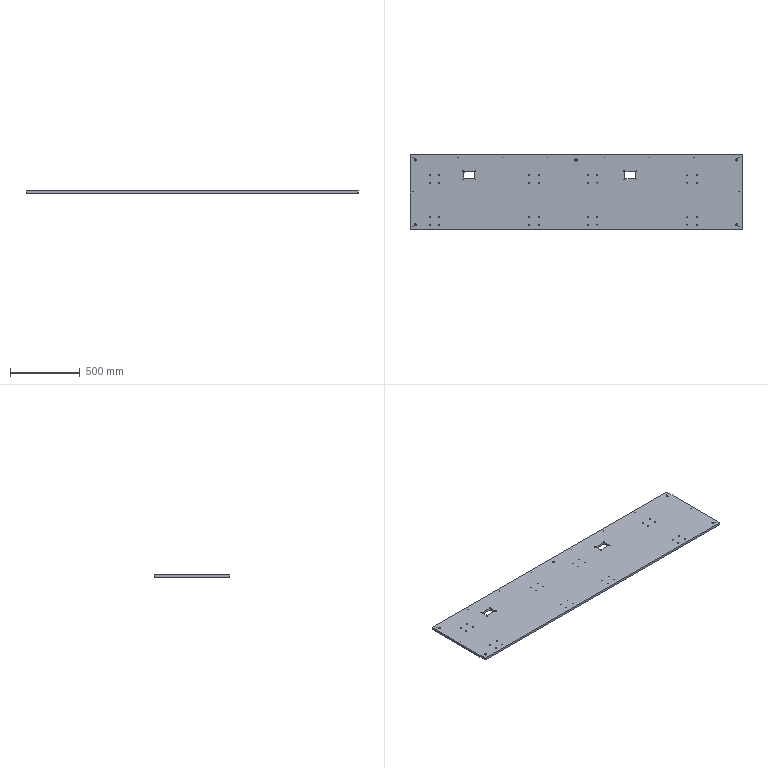Part | NX | features BREP 1 | 1 solid | 171 faces | box 2374 x 541 x 16 mm | volume 20391751 mm3 | cylinder 132 | plane 23 | cone 16 | commonest cylinder face diameters 7 x64 3.3 x40 9 x10 15 x10 20 x8